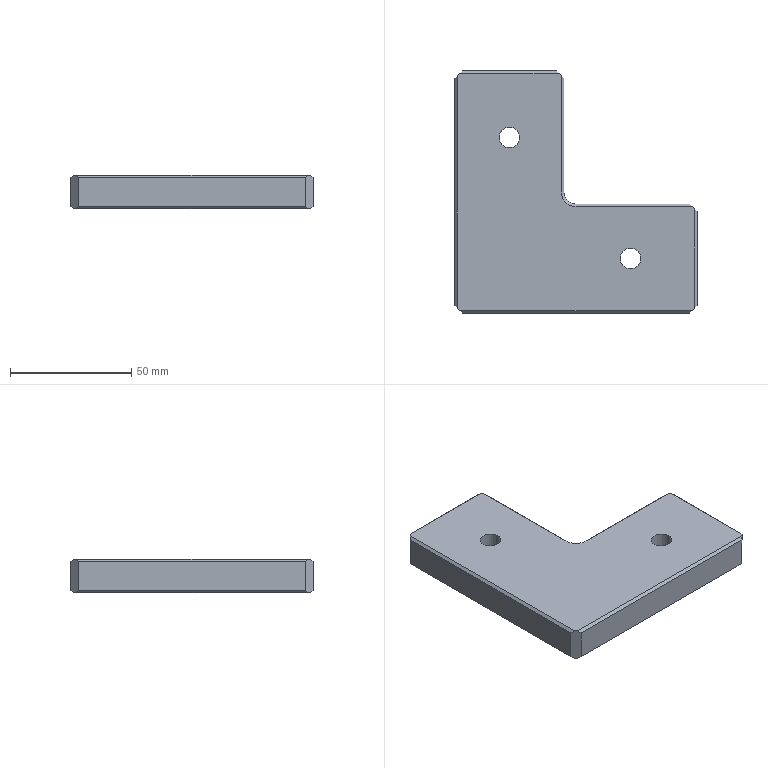Part | NX | 1 solid | 30 faces | box 100 x 100 x 14 mm | volume 95450 mm3 | plane 25 | cylinder 3 | cone 2 | commonest cylinder face diameters 8.5 x2 10 x1
STEP:
#1=CARTESIAN_POINT('',(42.,100.,1.));
#2=VERTEX_POINT('',#1);
#3=CARTESIAN_POINT('',(3.,100.,1.));
#4=VERTEX_POINT('',#3);
#5=CARTESIAN_POINT('',(45.,100.,1.));
#6=DIRECTION('',(-1.,0.,0.));
#7=VECTOR('',#6,1000.);
#8=LINE('',#5,#7);
#9=EDGE_CURVE('',#2,#4,#8,.T.);
#10=ORIENTED_EDGE('',*,*,#9,.T.);
#11=CARTESIAN_POINT('',(3.,100.,13.));
#12=VERTEX_POINT('',#11);
#13=CARTESIAN_POINT('',(3.,100.,14.));
#14=DIRECTION('',(0.,0.,1.));
#15=VECTOR('',#14,1000.);
#16=LINE('',#13,#15);
#17=EDGE_CURVE('',#4,#12,#16,.T.);
#18=ORIENTED_EDGE('',*,*,#17,.T.);
#19=CARTESIAN_POINT('',(42.,100.,13.));
#20=VERTEX_POINT('',#19);
#21=CARTESIAN_POINT('',(45.,100.,13.));
#22=DIRECTION('',(1.,0.,0.));
#23=VECTOR('',#22,1000.);
#24=LINE('',#21,#23);
#25=EDGE_CURVE('',#12,#20,#24,.T.);
#26=ORIENTED_EDGE('',*,*,#25,.T.);
#27=CARTESIAN_POINT('',(42.,100.,14.));
#28=DIRECTION('',(0.,0.,-1.));
#29=VECTOR('',#28,1000.);
#30=LINE('',#27,#29);
#31=EDGE_CURVE('',#20,#2,#30,.T.);
#32=ORIENTED_EDGE('',*,*,#31,.T.);
#33=EDGE_LOOP('',(#10,#18,#26,#32));
#34=FACE_BOUND('',#33,.T.);
#35=CARTESIAN_POINT('',(45.,100.,14.));
#36=DIRECTION('',(0.,-1.,0.));
#37=DIRECTION('',(0.,0.,-1.));
#38=AXIS2_PLACEMENT_3D('',#35,#36,#37);
#39=PLANE('',#38);
#40=ADVANCED_FACE('',(#34),#39,.F.);
#41=CARTESIAN_POINT('',(0.,3.,13.));
#42=VERTEX_POINT('',#41);
#43=CARTESIAN_POINT('',(0.,97.,13.));
#44=VERTEX_POINT('',#43);
#45=CARTESIAN_POINT('',(0.,100.,13.));
#46=DIRECTION('',(0.,1.,0.));
#47=VECTOR('',#46,1000.);
#48=LINE('',#45,#47);
#49=EDGE_CURVE('',#42,#44,#48,.T.);
#50=ORIENTED_EDGE('',*,*,#49,.T.);
#51=CARTESIAN_POINT('',(0.,97.,1.));
#52=VERTEX_POINT('',#51);
#53=CARTESIAN_POINT('',(0.,97.,14.));
#54=DIRECTION('',(0.,0.,-1.));
#55=VECTOR('',#54,1000.);
#56=LINE('',#53,#55);
#57=EDGE_CURVE('',#44,#52,#56,.T.);
#58=ORIENTED_EDGE('',*,*,#57,.T.);
#59=CARTESIAN_POINT('',(0.,3.,1.));
#60=VERTEX_POINT('',#59);
#61=CARTESIAN_POINT('',(0.,100.,1.));
#62=DIRECTION('',(0.,-1.,0.));
#63=VECTOR('',#62,1000.);
#64=LINE('',#61,#63);
#65=EDGE_CURVE('',#52,#60,#64,.T.);
#66=ORIENTED_EDGE('',*,*,#65,.T.);
#67=CARTESIAN_POINT('',(0.,3.,14.));
#68=DIRECTION('',(0.,0.,1.));
#69=VECTOR('',#68,1000.);
#70=LINE('',#67,#69);
#71=EDGE_CURVE('',#60,#42,#70,.T.);
#72=ORIENTED_EDGE('',*,*,#71,.T.);
#73=EDGE_LOOP('',(#50,#58,#66,#72));
#74=FACE_BOUND('',#73,.T.);
#75=CARTESIAN_POINT('',(0.,100.,14.));
#76=DIRECTION('',(1.,0.,0.));
#77=DIRECTION('',(0.,1.,0.));
#78=AXIS2_PLACEMENT_3D('',#75,#76,#77);
#79=PLANE('',#78);
#80=ADVANCED_FACE('',(#74),#79,.F.);
#81=CARTESIAN_POINT('',(3.,0.,1.));
#82=VERTEX_POINT('',#81);
#83=CARTESIAN_POINT('',(97.,0.,1.));
#84=VERTEX_POINT('',#83);
#85=CARTESIAN_POINT('',(0.,0.,1.));
#86=DIRECTION('',(1.,0.,0.));
#87=VECTOR('',#86,1000.);
#88=LINE('',#85,#87);
#89=EDGE_CURVE('',#82,#84,#88,.T.);
#90=ORIENTED_EDGE('',*,*,#89,.T.);
#91=CARTESIAN_POINT('',(97.,0.,13.));
#92=VERTEX_POINT('',#91);
#93=CARTESIAN_POINT('',(97.,0.,14.));
#94=DIRECTION('',(0.,0.,1.));
#95=VECTOR('',#94,1000.);
#96=LINE('',#93,#95);
#97=EDGE_CURVE('',#84,#92,#96,.T.);
#98=ORIENTED_EDGE('',*,*,#97,.T.);
#99=CARTESIAN_POINT('',(3.,0.,13.));
#100=VERTEX_POINT('',#99);
#101=CARTESIAN_POINT('',(0.,0.,13.));
#102=DIRECTION('',(-1.,0.,0.));
#103=VECTOR('',#102,1000.);
#104=LINE('',#101,#103);
#105=EDGE_CURVE('',#92,#100,#104,.T.);
#106=ORIENTED_EDGE('',*,*,#105,.T.);
#107=CARTESIAN_POINT('',(3.,0.,14.));
#108=DIRECTION('',(0.,0.,-1.));
#109=VECTOR('',#108,1000.);
#110=LINE('',#107,#109);
#111=EDGE_CURVE('',#100,#82,#110,.T.);
#112=ORIENTED_EDGE('',*,*,#111,.T.);
#113=EDGE_LOOP('',(#90,#98,#106,#112));
#114=FACE_BOUND('',#113,.T.);
#115=CARTESIAN_POINT('',(0.,0.,14.));
#116=DIRECTION('',(0.,1.,0.));
#117=DIRECTION('',(0.,0.,1.));
#118=AXIS2_PLACEMENT_3D('',#115,#116,#117);
#119=PLANE('',#118);
#120=ADVANCED_FACE('',(#114),#119,.F.);
#121=CARTESIAN_POINT('',(100.,3.,1.));
#122=VERTEX_POINT('',#121);
#123=CARTESIAN_POINT('',(100.,42.,1.));
#124=VERTEX_POINT('',#123);
#125=CARTESIAN_POINT('',(100.,0.,1.));
#126=DIRECTION('',(0.,1.,0.));
#127=VECTOR('',#126,1000.);
#128=LINE('',#125,#127);
#129=EDGE_CURVE('',#122,#124,#128,.T.);
#130=ORIENTED_EDGE('',*,*,#129,.T.);
#131=CARTESIAN_POINT('',(100.,42.,13.));
#132=VERTEX_POINT('',#131);
#133=CARTESIAN_POINT('',(100.,42.,14.));
#134=DIRECTION('',(0.,0.,1.));
#135=VECTOR('',#134,1000.);
#136=LINE('',#133,#135);
#137=EDGE_CURVE('',#124,#132,#136,.T.);
#138=ORIENTED_EDGE('',*,*,#137,.T.);
#139=CARTESIAN_POINT('',(100.,3.,13.));
#140=VERTEX_POINT('',#139);
#141=CARTESIAN_POINT('',(100.,0.,13.));
#142=DIRECTION('',(0.,-1.,0.));
#143=VECTOR('',#142,1000.);
#144=LINE('',#141,#143);
#145=EDGE_CURVE('',#132,#140,#144,.T.);
#146=ORIENTED_EDGE('',*,*,#145,.T.);
#147=CARTESIAN_POINT('',(100.,3.,14.));
#148=DIRECTION('',(0.,0.,-1.));
#149=VECTOR('',#148,1000.);
#150=LINE('',#147,#149);
#151=EDGE_CURVE('',#140,#122,#150,.T.);
#152=ORIENTED_EDGE('',*,*,#151,.T.);
#153=EDGE_LOOP('',(#130,#138,#146,#152));
#154=FACE_BOUND('',#153,.T.);
#155=CARTESIAN_POINT('',(100.,0.,14.));
#156=DIRECTION('',(-1.,0.,0.));
#157=DIRECTION('',(0.,0.,1.));
#158=AXIS2_PLACEMENT_3D('',#155,#156,#157);
#159=PLANE('',#158);
#160=ADVANCED_FACE('',(#154),#159,.F.);
#161=CARTESIAN_POINT('',(50.,45.,13.));
#162=VERTEX_POINT('',#161);
#163=CARTESIAN_POINT('',(97.,45.,13.));
#164=VERTEX_POINT('',#163);
#165=CARTESIAN_POINT('',(100.,45.,13.));
#166=DIRECTION('',(1.,0.,0.));
#167=VECTOR('',#166,1000.);
#168=LINE('',#165,#167);
#169=EDGE_CURVE('',#162,#164,#168,.T.);
#170=ORIENTED_EDGE('',*,*,#169,.T.);
#171=CARTESIAN_POINT('',(97.,45.,1.));
#172=VERTEX_POINT('',#171);
#173=CARTESIAN_POINT('',(97.,45.,14.));
#174=DIRECTION('',(0.,0.,-1.));
#175=VECTOR('',#174,1000.);
#176=LINE('',#173,#175);
#177=EDGE_CURVE('',#164,#172,#176,.T.);
#178=ORIENTED_EDGE('',*,*,#177,.T.);
#179=CARTESIAN_POINT('',(50.,45.,1.));
#180=VERTEX_POINT('',#179);
#181=CARTESIAN_POINT('',(100.,45.,1.));
#182=DIRECTION('',(-1.,0.,0.));
#183=VECTOR('',#182,1000.);
#184=LINE('',#181,#183);
#185=EDGE_CURVE('',#172,#180,#184,.T.);
#186=ORIENTED_EDGE('',*,*,#185,.T.);
#187=CARTESIAN_POINT('',(50.,45.,14.));
#188=DIRECTION('',(0.,0.,-1.));
#189=VECTOR('',#188,1000.);
#190=LINE('',#187,#189);
#191=EDGE_CURVE('',#180,#162,#190,.F.);
#192=ORIENTED_EDGE('',*,*,#191,.T.);
#193=EDGE_LOOP('',(#170,#178,#186,#192));
#194=FACE_BOUND('',#193,.T.);
#195=CARTESIAN_POINT('',(100.,45.,14.));
#196=DIRECTION('',(0.,-1.,0.));
#197=DIRECTION('',(0.,0.,-1.));
#198=AXIS2_PLACEMENT_3D('',#195,#196,#197);
#199=PLANE('',#198);
#200=ADVANCED_FACE('',(#194),#199,.F.);
#201=CARTESIAN_POINT('',(45.,50.,1.));
#202=VERTEX_POINT('',#201);
#203=CARTESIAN_POINT('',(45.,97.,1.));
#204=VERTEX_POINT('',#203);
#205=CARTESIAN_POINT('',(45.,45.,1.));
#206=DIRECTION('',(0.,1.,0.));
#207=VECTOR('',#206,1000.);
#208=LINE('',#205,#207);
#209=EDGE_CURVE('',#202,#204,#208,.T.);
#210=ORIENTED_EDGE('',*,*,#209,.T.);
#211=CARTESIAN_POINT('',(45.,97.,13.));
#212=VERTEX_POINT('',#211);
#213=CARTESIAN_POINT('',(45.,97.,14.));
#214=DIRECTION('',(0.,0.,1.));
#215=VECTOR('',#214,1000.);
#216=LINE('',#213,#215);
#217=EDGE_CURVE('',#204,#212,#216,.T.);
#218=ORIENTED_EDGE('',*,*,#217,.T.);
#219=CARTESIAN_POINT('',(45.,50.,13.));
#220=VERTEX_POINT('',#219);
#221=CARTESIAN_POINT('',(45.,50.,13.));
#222=DIRECTION('',(0.,-1.,0.));
#223=VECTOR('',#222,1000.);
#224=LINE('',#221,#223);
#225=EDGE_CURVE('',#212,#220,#224,.T.);
#226=ORIENTED_EDGE('',*,*,#225,.T.);
#227=CARTESIAN_POINT('',(45.,50.,0.));
#228=DIRECTION('',(0.,0.,-1.));
#229=VECTOR('',#228,1000.);
#230=LINE('',#227,#229);
#231=EDGE_CURVE('',#220,#202,#230,.T.);
#232=ORIENTED_EDGE('',*,*,#231,.T.);
#233=EDGE_LOOP('',(#210,#218,#226,#232));
#234=FACE_BOUND('',#233,.T.);
#235=CARTESIAN_POINT('',(45.,45.,14.));
#236=DIRECTION('',(-1.,0.,0.));
#237=DIRECTION('',(0.,-1.,0.));
#238=AXIS2_PLACEMENT_3D('',#235,#236,#237);
#239=PLANE('',#238);
#240=ADVANCED_FACE('',(#234),#239,.F.);
#241=CARTESIAN_POINT('',(26.75,72.5,14.));
#242=VERTEX_POINT('',#241);
#243=CARTESIAN_POINT('',(22.5,72.5,14.));
#244=DIRECTION('',(0.,0.,1.));
#245=DIRECTION('',(1.,0.,0.));
#246=AXIS2_PLACEMENT_3D('',#243,#244,#245);
#247=CIRCLE('',#246,4.25);
#248=EDGE_CURVE('',#242,#242,#247,.T.);
#249=ORIENTED_EDGE('',*,*,#248,.F.);
#250=EDGE_LOOP('',(#249));
#251=FACE_BOUND('',#250,.T.);
#252=CARTESIAN_POINT('',(76.75,22.5,14.));
#253=VERTEX_POINT('',#252);
#254=CARTESIAN_POINT('',(72.5,22.5,14.));
#255=DIRECTION('',(0.,0.,1.));
#256=DIRECTION('',(1.,0.,0.));
#257=AXIS2_PLACEMENT_3D('',#254,#255,#256);
#258=CIRCLE('',#257,4.25);
#259=EDGE_CURVE('',#253,#253,#258,.T.);
#260=ORIENTED_EDGE('',*,*,#259,.F.);
#261=EDGE_LOOP('',(#260));
#262=FACE_BOUND('',#261,.T.);
#263=CARTESIAN_POINT('',(43.,99.,14.));
#264=VERTEX_POINT('',#263);
#265=CARTESIAN_POINT('',(2.,99.,14.));
#266=VERTEX_POINT('',#265);
#267=CARTESIAN_POINT('',(0.,99.,14.));
#268=DIRECTION('',(-1.,0.,0.));
#269=VECTOR('',#268,1000.);
#270=LINE('',#267,#269);
#271=EDGE_CURVE('',#264,#266,#270,.T.);
#272=ORIENTED_EDGE('',*,*,#271,.T.);
#273=CARTESIAN_POINT('',(1.,98.,14.));
#274=VERTEX_POINT('',#273);
#275=CARTESIAN_POINT('',(-48.5,48.5,14.));
#276=DIRECTION('',(0.7071,0.7071,0.));
#277=VECTOR('',#276,1000.);
#278=LINE('',#275,#277);
#279=EDGE_CURVE('',#266,#274,#278,.F.);
#280=ORIENTED_EDGE('',*,*,#279,.T.);
#281=CARTESIAN_POINT('',(1.,2.,14.));
#282=VERTEX_POINT('',#281);
#283=CARTESIAN_POINT('',(1.,0.,14.));
#284=DIRECTION('',(0.,-1.,0.));
#285=VECTOR('',#284,1000.);
#286=LINE('',#283,#285);
#287=EDGE_CURVE('',#274,#282,#286,.T.);
#288=ORIENTED_EDGE('',*,*,#287,.T.);
#289=CARTESIAN_POINT('',(2.,1.,14.));
#290=VERTEX_POINT('',#289);
#291=CARTESIAN_POINT('',(1.5,1.5,14.));
#292=DIRECTION('',(-0.7071,0.7071,0.));
#293=VECTOR('',#292,1000.);
#294=LINE('',#291,#293);
#295=EDGE_CURVE('',#282,#290,#294,.F.);
#296=ORIENTED_EDGE('',*,*,#295,.T.);
#297=CARTESIAN_POINT('',(98.,1.,14.));
#298=VERTEX_POINT('',#297);
#299=CARTESIAN_POINT('',(100.,1.,14.));
#300=DIRECTION('',(1.,0.,0.));
#301=VECTOR('',#300,1000.);
#302=LINE('',#299,#301);
#303=EDGE_CURVE('',#290,#298,#302,.T.);
#304=ORIENTED_EDGE('',*,*,#303,.T.);
#305=CARTESIAN_POINT('',(99.,2.,14.));
#306=VERTEX_POINT('',#305);
#307=CARTESIAN_POINT('',(48.5,-48.5,14.));
#308=DIRECTION('',(-0.7071,-0.7071,0.));
#309=VECTOR('',#308,1000.);
#310=LINE('',#307,#309);
#311=EDGE_CURVE('',#298,#306,#310,.F.);
#312=ORIENTED_EDGE('',*,*,#311,.T.);
#313=CARTESIAN_POINT('',(99.,43.,14.));
#314=VERTEX_POINT('',#313);
#315=CARTESIAN_POINT('',(99.,45.,14.));
#316=DIRECTION('',(0.,1.,0.));
#317=VECTOR('',#316,1000.);
#318=LINE('',#315,#317);
#319=EDGE_CURVE('',#306,#314,#318,.T.);
#320=ORIENTED_EDGE('',*,*,#319,.T.);
#321=CARTESIAN_POINT('',(98.,44.,14.));
#322=VERTEX_POINT('',#321);
#323=CARTESIAN_POINT('',(71.,71.,14.));
#324=DIRECTION('',(0.7071,-0.7071,0.));
#325=VECTOR('',#324,1000.);
#326=LINE('',#323,#325);
#327=EDGE_CURVE('',#314,#322,#326,.F.);
#328=ORIENTED_EDGE('',*,*,#327,.T.);
#329=CARTESIAN_POINT('',(50.,44.,14.));
#330=VERTEX_POINT('',#329);
#331=CARTESIAN_POINT('',(50.,44.,14.));
#332=DIRECTION('',(-1.,0.,0.));
#333=VECTOR('',#332,1000.);
#334=LINE('',#331,#333);
#335=EDGE_CURVE('',#322,#330,#334,.T.);
#336=ORIENTED_EDGE('',*,*,#335,.T.);
#337=CARTESIAN_POINT('',(44.,50.,14.));
#338=VERTEX_POINT('',#337);
#339=CARTESIAN_POINT('',(50.,50.,14.));
#340=DIRECTION('',(0.,0.,1.));
#341=DIRECTION('',(1.,0.,0.));
#342=AXIS2_PLACEMENT_3D('',#339,#340,#341);
#343=CIRCLE('',#342,6.);
#344=EDGE_CURVE('',#330,#338,#343,.F.);
#345=ORIENTED_EDGE('',*,*,#344,.T.);
#346=CARTESIAN_POINT('',(44.,98.,14.));
#347=VERTEX_POINT('',#346);
#348=CARTESIAN_POINT('',(44.,100.,14.));
#349=DIRECTION('',(0.,1.,0.));
#350=VECTOR('',#349,1000.);
#351=LINE('',#348,#350);
#352=EDGE_CURVE('',#338,#347,#351,.T.);
#353=ORIENTED_EDGE('',*,*,#352,.T.);
#354=CARTESIAN_POINT('',(71.,71.,14.));
#355=DIRECTION('',(0.7071,-0.7071,0.));
#356=VECTOR('',#355,1000.);
#357=LINE('',#354,#356);
#358=EDGE_CURVE('',#347,#264,#357,.F.);
#359=ORIENTED_EDGE('',*,*,#358,.T.);
#360=EDGE_LOOP('',(#272,#280,#288,#296,#304,#312,#320,#328,#336,#345,#353,#359));
#361=FACE_BOUND('',#360,.T.);
#362=CARTESIAN_POINT('',(0.,0.,14.));
#363=DIRECTION('',(0.,0.,1.));
#364=DIRECTION('',(1.,0.,0.));
#365=AXIS2_PLACEMENT_3D('',#362,#363,#364);
#366=PLANE('',#365);
#367=ADVANCED_FACE('',(#251,#262,#361),#366,.T.);
#368=CARTESIAN_POINT('',(26.75,72.5,0.));
#369=VERTEX_POINT('',#368);
#370=CARTESIAN_POINT('',(22.5,72.5,0.));
#371=DIRECTION('',(0.,0.,1.));
#372=DIRECTION('',(1.,0.,0.));
#373=AXIS2_PLACEMENT_3D('',#370,#371,#372);
#374=CIRCLE('',#373,4.25);
#375=EDGE_CURVE('',#369,#369,#374,.T.);
#376=ORIENTED_EDGE('',*,*,#375,.T.);
#377=EDGE_LOOP('',(#376));
#378=FACE_BOUND('',#377,.T.);
#379=CARTESIAN_POINT('',(76.75,22.5,0.));
#380=VERTEX_POINT('',#379);
#381=CARTESIAN_POINT('',(72.5,22.5,0.));
#382=DIRECTION('',(0.,0.,1.));
#383=DIRECTION('',(1.,0.,0.));
#384=AXIS2_PLACEMENT_3D('',#381,#382,#383);
#385=CIRCLE('',#384,4.25);
#386=EDGE_CURVE('',#380,#380,#385,.T.);
#387=ORIENTED_EDGE('',*,*,#386,.T.);
#388=EDGE_LOOP('',(#387));
#389=FACE_BOUND('',#388,.T.);
#390=CARTESIAN_POINT('',(1.,2.,0.));
#391=VERTEX_POINT('',#390);
#392=CARTESIAN_POINT('',(1.,98.,0.));
#393=VERTEX_POINT('',#392);
#394=CARTESIAN_POINT('',(1.,0.,0.));
#395=DIRECTION('',(0.,1.,0.));
#396=VECTOR('',#395,1000.);
#397=LINE('',#394,#396);
#398=EDGE_CURVE('',#391,#393,#397,.T.);
#399=ORIENTED_EDGE('',*,*,#398,.T.);
#400=CARTESIAN_POINT('',(2.,99.,0.));
#401=VERTEX_POINT('',#400);
#402=CARTESIAN_POINT('',(0.,97.,0.));
#403=DIRECTION('',(-0.7071,-0.7071,0.));
#404=VECTOR('',#403,1000.);
#405=LINE('',#402,#404);
#406=EDGE_CURVE('',#393,#401,#405,.F.);
#407=ORIENTED_EDGE('',*,*,#406,.T.);
#408=CARTESIAN_POINT('',(43.,99.,0.));
#409=VERTEX_POINT('',#408);
#410=CARTESIAN_POINT('',(0.,99.,0.));
#411=DIRECTION('',(1.,0.,0.));
#412=VECTOR('',#411,1000.);
#413=LINE('',#410,#412);
#414=EDGE_CURVE('',#401,#409,#413,.T.);
#415=ORIENTED_EDGE('',*,*,#414,.T.);
#416=CARTESIAN_POINT('',(44.,98.,0.));
#417=VERTEX_POINT('',#416);
#418=CARTESIAN_POINT('',(42.,100.,0.));
#419=DIRECTION('',(-0.7071,0.7071,0.));
#420=VECTOR('',#419,1000.);
#421=LINE('',#418,#420);
#422=EDGE_CURVE('',#409,#417,#421,.F.);
#423=ORIENTED_EDGE('',*,*,#422,.T.);
#424=CARTESIAN_POINT('',(44.,50.,0.));
#425=VERTEX_POINT('',#424);
#426=CARTESIAN_POINT('',(44.,0.,0.));
#427=DIRECTION('',(0.,-1.,0.));
#428=VECTOR('',#427,1000.);
#429=LINE('',#426,#428);
#430=EDGE_CURVE('',#417,#425,#429,.T.);
#431=ORIENTED_EDGE('',*,*,#430,.T.);
#432=CARTESIAN_POINT('',(50.,44.,0.));
#433=VERTEX_POINT('',#432);
#434=CARTESIAN_POINT('',(50.,50.,0.));
#435=DIRECTION('',(0.,0.,1.));
#436=DIRECTION('',(1.,0.,0.));
#437=AXIS2_PLACEMENT_3D('',#434,#435,#436);
#438=CIRCLE('',#437,6.);
#439=EDGE_CURVE('',#425,#433,#438,.T.);
#440=ORIENTED_EDGE('',*,*,#439,.T.);
#441=CARTESIAN_POINT('',(98.,44.,0.));
#442=VERTEX_POINT('',#441);
#443=CARTESIAN_POINT('',(0.,44.,0.));
#444=DIRECTION('',(1.,0.,0.));
#445=VECTOR('',#444,1000.);
#446=LINE('',#443,#445);
#447=EDGE_CURVE('',#433,#442,#446,.T.);
#448=ORIENTED_EDGE('',*,*,#447,.T.);
#449=CARTESIAN_POINT('',(99.,43.,0.));
#450=VERTEX_POINT('',#449);
#451=CARTESIAN_POINT('',(97.,45.,0.));
#452=DIRECTION('',(-0.7071,0.7071,0.));
#453=VECTOR('',#452,1000.);
#454=LINE('',#451,#453);
#455=EDGE_CURVE('',#442,#450,#454,.F.);
#456=ORIENTED_EDGE('',*,*,#455,.T.);
#457=CARTESIAN_POINT('',(99.,2.,0.));
#458=VERTEX_POINT('',#457);
#459=CARTESIAN_POINT('',(99.,0.,0.));
#460=DIRECTION('',(0.,-1.,0.));
#461=VECTOR('',#460,1000.);
#462=LINE('',#459,#461);
#463=EDGE_CURVE('',#450,#458,#462,.T.);
#464=ORIENTED_EDGE('',*,*,#463,.T.);
#465=CARTESIAN_POINT('',(98.,1.,0.));
#466=VERTEX_POINT('',#465);
#467=CARTESIAN_POINT('',(100.,3.,0.));
#468=DIRECTION('',(0.7071,0.7071,0.));
#469=VECTOR('',#468,1000.);
#470=LINE('',#467,#469);
#471=EDGE_CURVE('',#458,#466,#470,.F.);
#472=ORIENTED_EDGE('',*,*,#471,.T.);
#473=CARTESIAN_POINT('',(2.,1.,0.));
#474=VERTEX_POINT('',#473);
#475=CARTESIAN_POINT('',(0.,1.,0.));
#476=DIRECTION('',(-1.,0.,0.));
#477=VECTOR('',#476,1000.);
#478=LINE('',#475,#477);
#479=EDGE_CURVE('',#466,#474,#478,.T.);
#480=ORIENTED_EDGE('',*,*,#479,.T.);
#481=CARTESIAN_POINT('',(3.,0.,0.));
#482=DIRECTION('',(0.7071,-0.7071,0.));
#483=VECTOR('',#482,1000.);
#484=LINE('',#481,#483);
#485=EDGE_CURVE('',#474,#391,#484,.F.);
#486=ORIENTED_EDGE('',*,*,#485,.T.);
#487=EDGE_LOOP('',(#399,#407,#415,#423,#431,#440,#448,#456,#464,#472,#480,#486));
#488=FACE_BOUND('',#487,.T.);
#489=CARTESIAN_POINT('',(0.,0.,0.));
#490=DIRECTION('',(0.,0.,1.));
#491=DIRECTION('',(1.,0.,0.));
#492=AXIS2_PLACEMENT_3D('',#489,#490,#491);
#493=PLANE('',#492);
#494=ADVANCED_FACE('',(#378,#389,#488),#493,.F.);
#495=ORIENTED_EDGE('',*,*,#191,.F.);
#496=CARTESIAN_POINT('',(50.,50.,1.));
#497=DIRECTION('',(0.,0.,1.));
#498=DIRECTION('',(1.,0.,0.));
#499=AXIS2_PLACEMENT_3D('',#496,#497,#498);
#500=CIRCLE('',#499,5.);
#501=EDGE_CURVE('',#180,#202,#500,.F.);
#502=ORIENTED_EDGE('',*,*,#501,.T.);
#503=ORIENTED_EDGE('',*,*,#231,.F.);
#504=CARTESIAN_POINT('',(50.,50.,13.));
#505=DIRECTION('',(0.,0.,1.));
#506=DIRECTION('',(1.,0.,0.));
#507=AXIS2_PLACEMENT_3D('',#504,#505,#506);
#508=CIRCLE('',#507,5.);
#509=EDGE_CURVE('',#220,#162,#508,.T.);
#510=ORIENTED_EDGE('',*,*,#509,.T.);
#511=EDGE_LOOP('',(#495,#502,#503,#510));
#512=FACE_BOUND('',#511,.T.);
#513=CARTESIAN_POINT('',(50.,50.,14.));
#514=DIRECTION('',(0.,0.,1.));
#515=DIRECTION('',(1.,0.,0.));
#516=AXIS2_PLACEMENT_3D('',#513,#514,#515);
#517=CYLINDRICAL_SURFACE('',#516,5.);
#518=ADVANCED_FACE('',(#512),#517,.F.);
#519=ORIENTED_EDGE('',*,*,#65,.F.);
#520=CARTESIAN_POINT('',(1.,98.,0.));
#521=DIRECTION('',(0.5774,0.5774,-0.5774));
#522=VECTOR('',#521,1000.);
#523=LINE('',#520,#522);
#524=EDGE_CURVE('',#52,#393,#523,.T.);
#525=ORIENTED_EDGE('',*,*,#524,.T.);
#526=ORIENTED_EDGE('',*,*,#398,.F.);
#527=CARTESIAN_POINT('',(-32.333,35.333,33.333));
#528=DIRECTION('',(-0.5774,0.5774,0.5774));
#529=VECTOR('',#528,1000.);
#530=LINE('',#527,#529);
#531=EDGE_CURVE('',#391,#60,#530,.T.);
#532=ORIENTED_EDGE('',*,*,#531,.T.);
#533=EDGE_LOOP('',(#519,#525,#526,#532));
#534=FACE_BOUND('',#533,.T.);
#535=CARTESIAN_POINT('',(0.,100.,1.));
#536=DIRECTION('',(0.7071,0.,0.7071));
#537=DIRECTION('',(0.,-1.,0.));
#538=AXIS2_PLACEMENT_3D('',#535,#536,#537);
#539=PLANE('',#538);
#540=ADVANCED_FACE('',(#534),#539,.F.);
#541=ORIENTED_EDGE('',*,*,#479,.F.);
#542=CARTESIAN_POINT('',(64.667,-32.333,33.333));
#543=DIRECTION('',(-0.5774,-0.5774,0.5774));
#544=VECTOR('',#543,1000.);
#545=LINE('',#542,#544);
#546=EDGE_CURVE('',#466,#84,#545,.T.);
#547=ORIENTED_EDGE('',*,*,#546,.T.);
#548=ORIENTED_EDGE('',*,*,#89,.F.);
#549=CARTESIAN_POINT('',(2.,1.,0.));
#550=DIRECTION('',(-0.5774,0.5774,-0.5774));
#551=VECTOR('',#550,1000.);
#552=LINE('',#549,#551);
#553=EDGE_CURVE('',#82,#474,#552,.T.);
#554=ORIENTED_EDGE('',*,*,#553,.T.);
#555=EDGE_LOOP('',(#541,#547,#548,#554));
#556=FACE_BOUND('',#555,.T.);
#557=CARTESIAN_POINT('',(0.,0.,1.));
#558=DIRECTION('',(0.,0.7071,0.7071));
#559=DIRECTION('',(1.,0.,0.));
#560=AXIS2_PLACEMENT_3D('',#557,#558,#559);
#561=PLANE('',#560);
#562=ADVANCED_FACE('',(#556),#561,.F.);
#563=ORIENTED_EDGE('',*,*,#414,.F.);
#564=CARTESIAN_POINT('',(17.,114.,15.));
#565=DIRECTION('',(0.5774,0.5774,0.5774));
#566=VECTOR('',#565,1000.);
#567=LINE('',#564,#566);
#568=EDGE_CURVE('',#401,#4,#567,.T.);
#569=ORIENTED_EDGE('',*,*,#568,.T.);
#570=ORIENTED_EDGE('',*,*,#9,.F.);
#571=CARTESIAN_POINT('',(43.,99.,0.));
#572=DIRECTION('',(0.5774,-0.5774,-0.5774));
#573=VECTOR('',#572,1000.);
#574=LINE('',#571,#573);
#575=EDGE_CURVE('',#2,#409,#574,.T.);
#576=ORIENTED_EDGE('',*,*,#575,.T.);
#577=EDGE_LOOP('',(#563,#569,#570,#576));
#578=FACE_BOUND('',#577,.T.);
#579=CARTESIAN_POINT('',(45.,100.,1.));
#580=DIRECTION('',(0.,-0.7071,0.7071));
#581=DIRECTION('',(-1.,0.,0.));
#582=AXIS2_PLACEMENT_3D('',#579,#580,#581);
#583=PLANE('',#582);
#584=ADVANCED_FACE('',(#578),#583,.F.);
#585=ORIENTED_EDGE('',*,*,#463,.F.);
#586=CARTESIAN_POINT('',(114.,28.,15.));
#587=DIRECTION('',(0.5774,-0.5774,0.5774));
#588=VECTOR('',#587,1000.);
#589=LINE('',#586,#588);
#590=EDGE_CURVE('',#450,#124,#589,.T.);
#591=ORIENTED_EDGE('',*,*,#590,.T.);
#592=ORIENTED_EDGE('',*,*,#129,.F.);
#593=CARTESIAN_POINT('',(99.,2.,0.));
#594=DIRECTION('',(-0.5774,-0.5774,-0.5774));
#595=VECTOR('',#594,1000.);
#596=LINE('',#593,#595);
#597=EDGE_CURVE('',#122,#458,#596,.T.);
#598=ORIENTED_EDGE('',*,*,#597,.T.);
#599=EDGE_LOOP('',(#585,#591,#592,#598));
#600=FACE_BOUND('',#599,.T.);
#601=CARTESIAN_POINT('',(100.,0.,1.));
#602=DIRECTION('',(-0.7071,0.,0.7071));
#603=DIRECTION('',(0.,1.,0.));
#604=AXIS2_PLACEMENT_3D('',#601,#602,#603);
#605=PLANE('',#604);
#606=ADVANCED_FACE('',(#600),#605,.F.);
#607=ORIENTED_EDGE('',*,*,#430,.F.);
#608=CARTESIAN_POINT('',(62.333,79.667,18.333));
#609=DIRECTION('',(0.5774,-0.5774,0.5774));
#610=VECTOR('',#609,1000.);
#611=LINE('',#608,#610);
#612=EDGE_CURVE('',#417,#204,#611,.T.);
#613=ORIENTED_EDGE('',*,*,#612,.T.);
#614=ORIENTED_EDGE('',*,*,#209,.F.);
#615=CARTESIAN_POINT('',(44.,50.,0.));
#616=DIRECTION('',(0.7071,0.,0.7071));
#617=VECTOR('',#616,1000.);
#618=LINE('',#615,#617);
#619=EDGE_CURVE('',#425,#202,#618,.T.);
#620=ORIENTED_EDGE('',*,*,#619,.F.);
#621=EDGE_LOOP('',(#607,#613,#614,#620));
#622=FACE_BOUND('',#621,.T.);
#623=CARTESIAN_POINT('',(45.,45.,1.));
#624=DIRECTION('',(-0.7071,0.,0.7071));
#625=DIRECTION('',(0.,1.,0.));
#626=AXIS2_PLACEMENT_3D('',#623,#624,#625);
#627=PLANE('',#626);
#628=ADVANCED_FACE('',(#622),#627,.F.);
#629=ORIENTED_EDGE('',*,*,#185,.F.);
#630=CARTESIAN_POINT('',(98.,44.,0.));
#631=DIRECTION('',(0.5774,-0.5774,-0.5774));
#632=VECTOR('',#631,1000.);
#633=LINE('',#630,#632);
#634=EDGE_CURVE('',#172,#442,#633,.T.);
#635=ORIENTED_EDGE('',*,*,#634,.T.);
#636=ORIENTED_EDGE('',*,*,#447,.F.);
#637=CARTESIAN_POINT('',(50.,45.,1.));
#638=DIRECTION('',(0.,-0.7071,-0.7071));
#639=VECTOR('',#638,1000.);
#640=LINE('',#637,#639);
#641=EDGE_CURVE('',#180,#433,#640,.T.);
#642=ORIENTED_EDGE('',*,*,#641,.F.);
#643=EDGE_LOOP('',(#629,#635,#636,#642));
#644=FACE_BOUND('',#643,.T.);
#645=CARTESIAN_POINT('',(100.,45.,1.));
#646=DIRECTION('',(0.,-0.7071,0.7071));
#647=DIRECTION('',(-1.,0.,0.));
#648=AXIS2_PLACEMENT_3D('',#645,#646,#647);
#649=PLANE('',#648);
#650=ADVANCED_FACE('',(#644),#649,.F.);
#651=ORIENTED_EDGE('',*,*,#619,.T.);
#652=ORIENTED_EDGE('',*,*,#501,.F.);
#653=ORIENTED_EDGE('',*,*,#641,.T.);
#654=ORIENTED_EDGE('',*,*,#439,.F.);
#655=EDGE_LOOP('',(#651,#652,#653,#654));
#656=FACE_BOUND('',#655,.T.);
#657=CARTESIAN_POINT('',(50.,50.,0.));
#658=DIRECTION('',(0.,0.,-1.));
#659=DIRECTION('',(-1.,0.,0.));
#660=AXIS2_PLACEMENT_3D('',#657,#658,#659);
#661=CONICAL_SURFACE('',#660,6.,0.7854);
#662=ADVANCED_FACE('',(#656),#661,.F.);
#663=ORIENTED_EDGE('',*,*,#105,.F.);
#664=CARTESIAN_POINT('',(65.333,-31.667,-18.667));
#665=DIRECTION('',(-0.5774,-0.5774,-0.5774));
#666=VECTOR('',#665,1000.);
#667=LINE('',#664,#666);
#668=EDGE_CURVE('',#92,#298,#667,.F.);
#669=ORIENTED_EDGE('',*,*,#668,.T.);
#670=ORIENTED_EDGE('',*,*,#303,.F.);
#671=CARTESIAN_POINT('',(1.333,1.667,14.667));
#672=DIRECTION('',(-0.5774,0.5774,0.5774));
#673=VECTOR('',#672,1000.);
#674=LINE('',#671,#673);
#675=EDGE_CURVE('',#290,#100,#674,.F.);
#676=ORIENTED_EDGE('',*,*,#675,.T.);
#677=EDGE_LOOP('',(#663,#669,#670,#676));
#678=FACE_BOUND('',#677,.T.);
#679=CARTESIAN_POINT('',(0.,1.,14.));
#680=DIRECTION('',(0.,-0.7071,0.7071));
#681=DIRECTION('',(-1.,0.,0.));
#682=AXIS2_PLACEMENT_3D('',#679,#680,#681);
#683=PLANE('',#682);
#684=ADVANCED_FACE('',(#678),#683,.T.);
#685=ORIENTED_EDGE('',*,*,#287,.F.);
#686=CARTESIAN_POINT('',(-31.667,65.333,-18.667));
#687=DIRECTION('',(0.5774,0.5774,0.5774));
#688=VECTOR('',#687,1000.);
#689=LINE('',#686,#688);
#690=EDGE_CURVE('',#274,#44,#689,.F.);
#691=ORIENTED_EDGE('',*,*,#690,.T.);
#692=ORIENTED_EDGE('',*,*,#49,.F.);
#693=CARTESIAN_POINT('',(1.667,1.333,14.667));
#694=DIRECTION('',(-0.5774,0.5774,-0.5774));
#695=VECTOR('',#694,1000.);
#696=LINE('',#693,#695);
#697=EDGE_CURVE('',#42,#282,#696,.F.);
#698=ORIENTED_EDGE('',*,*,#697,.T.);
#699=EDGE_LOOP('',(#685,#691,#692,#698));
#700=FACE_BOUND('',#699,.T.);
#701=CARTESIAN_POINT('',(1.,0.,14.));
#702=DIRECTION('',(-0.7071,0.,0.7071));
#703=DIRECTION('',(0.,1.,0.));
#704=AXIS2_PLACEMENT_3D('',#701,#702,#703);
#705=PLANE('',#704);
#706=ADVANCED_FACE('',(#700),#705,.T.);
#707=ORIENTED_EDGE('',*,*,#145,.F.);
#708=CARTESIAN_POINT('',(113.333,28.667,-0.3333));
#709=DIRECTION('',(0.5774,-0.5774,-0.5774));
#710=VECTOR('',#709,1000.);
#711=LINE('',#708,#710);
#712=EDGE_CURVE('',#132,#314,#711,.F.);
#713=ORIENTED_EDGE('',*,*,#712,.T.);
#714=ORIENTED_EDGE('',*,*,#319,.F.);
#715=CARTESIAN_POINT('',(98.333,1.333,14.667));
#716=DIRECTION('',(-0.5774,-0.5774,0.5774));
#717=VECTOR('',#716,1000.);
#718=LINE('',#715,#717);
#719=EDGE_CURVE('',#306,#140,#718,.F.);
#720=ORIENTED_EDGE('',*,*,#719,.T.);
#721=EDGE_LOOP('',(#707,#713,#714,#720));
#722=FACE_BOUND('',#721,.T.);
#723=CARTESIAN_POINT('',(99.,0.,14.));
#724=DIRECTION('',(0.7071,0.,0.7071));
#725=DIRECTION('',(0.,-1.,0.));
#726=AXIS2_PLACEMENT_3D('',#723,#724,#725);
#727=PLANE('',#726);
#728=ADVANCED_FACE('',(#722),#727,.T.);
#729=ORIENTED_EDGE('',*,*,#25,.F.);
#730=CARTESIAN_POINT('',(1.333,98.333,14.667));
#731=DIRECTION('',(0.5774,0.5774,-0.5774));
#732=VECTOR('',#731,1000.);
#733=LINE('',#730,#732);
#734=EDGE_CURVE('',#12,#266,#733,.F.);
#735=ORIENTED_EDGE('',*,*,#734,.T.);
#736=ORIENTED_EDGE('',*,*,#271,.F.);
#737=CARTESIAN_POINT('',(28.667,113.333,-0.3333));
#738=DIRECTION('',(0.5774,-0.5774,0.5774));
#739=VECTOR('',#738,1000.);
#740=LINE('',#737,#739);
#741=EDGE_CURVE('',#264,#20,#740,.F.);
#742=ORIENTED_EDGE('',*,*,#741,.T.);
#743=EDGE_LOOP('',(#729,#735,#736,#742));
#744=FACE_BOUND('',#743,.T.);
#745=CARTESIAN_POINT('',(0.,99.,14.));
#746=DIRECTION('',(0.,0.7071,0.7071));
#747=DIRECTION('',(1.,0.,0.));
#748=AXIS2_PLACEMENT_3D('',#745,#746,#747);
#749=PLANE('',#748);
#750=ADVANCED_FACE('',(#744),#749,.T.);
#751=ORIENTED_EDGE('',*,*,#335,.F.);
#752=CARTESIAN_POINT('',(65.333,76.667,-18.667));
#753=DIRECTION('',(0.5774,-0.5774,0.5774));
#754=VECTOR('',#753,1000.);
#755=LINE('',#752,#754);
#756=EDGE_CURVE('',#322,#164,#755,.F.);
#757=ORIENTED_EDGE('',*,*,#756,.T.);
#758=ORIENTED_EDGE('',*,*,#169,.F.);
#759=CARTESIAN_POINT('',(50.,44.,14.));
#760=DIRECTION('',(0.,0.7071,-0.7071));
#761=VECTOR('',#760,1000.);
#762=LINE('',#759,#761);
#763=EDGE_CURVE('',#330,#162,#762,.T.);
#764=ORIENTED_EDGE('',*,*,#763,.F.);
#765=EDGE_LOOP('',(#751,#757,#758,#764));
#766=FACE_BOUND('',#765,.T.);
#767=CARTESIAN_POINT('',(0.,44.,14.));
#768=DIRECTION('',(0.,0.7071,0.7071));
#769=DIRECTION('',(1.,0.,0.));
#770=AXIS2_PLACEMENT_3D('',#767,#768,#769);
#771=PLANE('',#770);
#772=ADVANCED_FACE('',(#766),#771,.T.);
#773=ORIENTED_EDGE('',*,*,#225,.F.);
#774=CARTESIAN_POINT('',(76.667,65.333,-18.667));
#775=DIRECTION('',(0.5774,-0.5774,-0.5774));
#776=VECTOR('',#775,1000.);
#777=LINE('',#774,#776);
#778=EDGE_CURVE('',#212,#347,#777,.F.);
#779=ORIENTED_EDGE('',*,*,#778,.T.);
#780=ORIENTED_EDGE('',*,*,#352,.F.);
#781=CARTESIAN_POINT('',(45.,50.,13.));
#782=DIRECTION('',(-0.7071,0.,0.7071));
#783=VECTOR('',#782,1000.);
#784=LINE('',#781,#783);
#785=EDGE_CURVE('',#220,#338,#784,.T.);
#786=ORIENTED_EDGE('',*,*,#785,.F.);
#787=EDGE_LOOP('',(#773,#779,#780,#786));
#788=FACE_BOUND('',#787,.T.);
#789=CARTESIAN_POINT('',(44.,0.,14.));
#790=DIRECTION('',(0.7071,0.,0.7071));
#791=DIRECTION('',(0.,-1.,0.));
#792=AXIS2_PLACEMENT_3D('',#789,#790,#791);
#793=PLANE('',#792);
#794=ADVANCED_FACE('',(#788),#793,.T.);
#795=ORIENTED_EDGE('',*,*,#763,.T.);
#796=ORIENTED_EDGE('',*,*,#509,.F.);
#797=ORIENTED_EDGE('',*,*,#785,.T.);
#798=ORIENTED_EDGE('',*,*,#344,.F.);
#799=EDGE_LOOP('',(#795,#796,#797,#798));
#800=FACE_BOUND('',#799,.T.);
#801=CARTESIAN_POINT('',(50.,50.,14.));
#802=DIRECTION('',(0.,0.,1.));
#803=DIRECTION('',(1.,0.,0.));
#804=AXIS2_PLACEMENT_3D('',#801,#802,#803);
#805=CONICAL_SURFACE('',#804,6.,0.7854);
#806=ADVANCED_FACE('',(#800),#805,.F.);
#807=ORIENTED_EDGE('',*,*,#734,.F.);
#808=ORIENTED_EDGE('',*,*,#17,.F.);
#809=ORIENTED_EDGE('',*,*,#568,.F.);
#810=ORIENTED_EDGE('',*,*,#406,.F.);
#811=ORIENTED_EDGE('',*,*,#524,.F.);
#812=ORIENTED_EDGE('',*,*,#57,.F.);
#813=ORIENTED_EDGE('',*,*,#690,.F.);
#814=ORIENTED_EDGE('',*,*,#279,.F.);
#815=EDGE_LOOP('',(#807,#808,#809,#810,#811,#812,#813,#814));
#816=FACE_BOUND('',#815,.T.);
#817=CARTESIAN_POINT('',(0.,97.,14.));
#818=DIRECTION('',(0.7071,-0.7071,0.));
#819=DIRECTION('',(0.,0.,-1.));
#820=AXIS2_PLACEMENT_3D('',#817,#818,#819);
#821=PLANE('',#820);
#822=ADVANCED_FACE('',(#816),#821,.F.);
#823=ORIENTED_EDGE('',*,*,#778,.F.);
#824=ORIENTED_EDGE('',*,*,#217,.F.);
#825=ORIENTED_EDGE('',*,*,#612,.F.);
#826=ORIENTED_EDGE('',*,*,#422,.F.);
#827=ORIENTED_EDGE('',*,*,#575,.F.);
#828=ORIENTED_EDGE('',*,*,#31,.F.);
#829=ORIENTED_EDGE('',*,*,#741,.F.);
#830=ORIENTED_EDGE('',*,*,#358,.F.);
#831=EDGE_LOOP('',(#823,#824,#825,#826,#827,#828,#829,#830));
#832=FACE_BOUND('',#831,.T.);
#833=CARTESIAN_POINT('',(42.,100.,14.));
#834=DIRECTION('',(-0.7071,-0.7071,0.));
#835=DIRECTION('',(0.,0.,-1.));
#836=AXIS2_PLACEMENT_3D('',#833,#834,#835);
#837=PLANE('',#836);
#838=ADVANCED_FACE('',(#832),#837,.F.);
#839=ORIENTED_EDGE('',*,*,#712,.F.);
#840=ORIENTED_EDGE('',*,*,#137,.F.);
#841=ORIENTED_EDGE('',*,*,#590,.F.);
#842=ORIENTED_EDGE('',*,*,#455,.F.);
#843=ORIENTED_EDGE('',*,*,#634,.F.);
#844=ORIENTED_EDGE('',*,*,#177,.F.);
#845=ORIENTED_EDGE('',*,*,#756,.F.);
#846=ORIENTED_EDGE('',*,*,#327,.F.);
#847=EDGE_LOOP('',(#839,#840,#841,#842,#843,#844,#845,#846));
#848=FACE_BOUND('',#847,.T.);
#849=CARTESIAN_POINT('',(97.,45.,14.));
#850=DIRECTION('',(-0.7071,-0.7071,0.));
#851=DIRECTION('',(0.,0.,-1.));
#852=AXIS2_PLACEMENT_3D('',#849,#850,#851);
#853=PLANE('',#852);
#854=ADVANCED_FACE('',(#848),#853,.F.);
#855=ORIENTED_EDGE('',*,*,#668,.F.);
#856=ORIENTED_EDGE('',*,*,#97,.F.);
#857=ORIENTED_EDGE('',*,*,#546,.F.);
#858=ORIENTED_EDGE('',*,*,#471,.F.);
#859=ORIENTED_EDGE('',*,*,#597,.F.);
#860=ORIENTED_EDGE('',*,*,#151,.F.);
#861=ORIENTED_EDGE('',*,*,#719,.F.);
#862=ORIENTED_EDGE('',*,*,#311,.F.);
#863=EDGE_LOOP('',(#855,#856,#857,#858,#859,#860,#861,#862));
#864=FACE_BOUND('',#863,.T.);
#865=CARTESIAN_POINT('',(100.,3.,14.));
#866=DIRECTION('',(-0.7071,0.7071,0.));
#867=DIRECTION('',(0.,0.,-1.));
#868=AXIS2_PLACEMENT_3D('',#865,#866,#867);
#869=PLANE('',#868);
#870=ADVANCED_FACE('',(#864),#869,.F.);
#871=ORIENTED_EDGE('',*,*,#697,.F.);
#872=ORIENTED_EDGE('',*,*,#71,.F.);
#873=ORIENTED_EDGE('',*,*,#531,.F.);
#874=ORIENTED_EDGE('',*,*,#485,.F.);
#875=ORIENTED_EDGE('',*,*,#553,.F.);
#876=ORIENTED_EDGE('',*,*,#111,.F.);
#877=ORIENTED_EDGE('',*,*,#675,.F.);
#878=ORIENTED_EDGE('',*,*,#295,.F.);
#879=EDGE_LOOP('',(#871,#872,#873,#874,#875,#876,#877,#878));
#880=FACE_BOUND('',#879,.T.);
#881=CARTESIAN_POINT('',(3.,0.,14.));
#882=DIRECTION('',(0.7071,0.7071,0.));
#883=DIRECTION('',(0.,0.,-1.));
#884=AXIS2_PLACEMENT_3D('',#881,#882,#883);
#885=PLANE('',#884);
#886=ADVANCED_FACE('',(#880),#885,.F.);
#887=ORIENTED_EDGE('',*,*,#386,.F.);
#888=EDGE_LOOP('',(#887));
#889=FACE_BOUND('',#888,.T.);
#890=ORIENTED_EDGE('',*,*,#259,.T.);
#891=EDGE_LOOP('',(#890));
#892=FACE_BOUND('',#891,.T.);
#893=CARTESIAN_POINT('',(72.5,22.5,14.));
#894=DIRECTION('',(0.,0.,1.));
#895=DIRECTION('',(1.,0.,0.));
#896=AXIS2_PLACEMENT_3D('',#893,#894,#895);
#897=CYLINDRICAL_SURFACE('',#896,4.25);
#898=ADVANCED_FACE('',(#889,#892),#897,.F.);
#899=ORIENTED_EDGE('',*,*,#375,.F.);
#900=EDGE_LOOP('',(#899));
#901=FACE_BOUND('',#900,.T.);
#902=ORIENTED_EDGE('',*,*,#248,.T.);
#903=EDGE_LOOP('',(#902));
#904=FACE_BOUND('',#903,.T.);
#905=CARTESIAN_POINT('',(22.5,72.5,14.));
#906=DIRECTION('',(0.,0.,1.));
#907=DIRECTION('',(1.,0.,0.));
#908=AXIS2_PLACEMENT_3D('',#905,#906,#907);
#909=CYLINDRICAL_SURFACE('',#908,4.25);
#910=ADVANCED_FACE('',(#901,#904),#909,.F.);
#911=CLOSED_SHELL('',(#40,#80,#120,#160,#200,#240,#367,#494,#518,#540,#562,#584,#606,#628,#650,#662,#684,#706,#728,#750,#772,#794,#806,#822,#838,#854,#870,#886,#898,#910));
#912=MANIFOLD_SOLID_BREP('',#911);
#913=(LENGTH_UNIT()NAMED_UNIT(*)SI_UNIT(.MILLI.,.METRE.));
#914=UNCERTAINTY_MEASURE_WITH_UNIT(LENGTH_MEASURE(0.00001),#913,'','');
#915=(NAMED_UNIT(*)PLANE_ANGLE_UNIT()SI_UNIT($,.RADIAN.));
#916=(NAMED_UNIT(*)SI_UNIT($,.STERADIAN.)SOLID_ANGLE_UNIT());
#917=(GEOMETRIC_REPRESENTATION_CONTEXT(3)GLOBAL_UNCERTAINTY_ASSIGNED_CONTEXT((#914))GLOBAL_UNIT_ASSIGNED_CONTEXT((#913,#915,#916))REPRESENTATION_CONTEXT('',''));
#918=ADVANCED_BREP_SHAPE_REPRESENTATION('',(#912),#917);